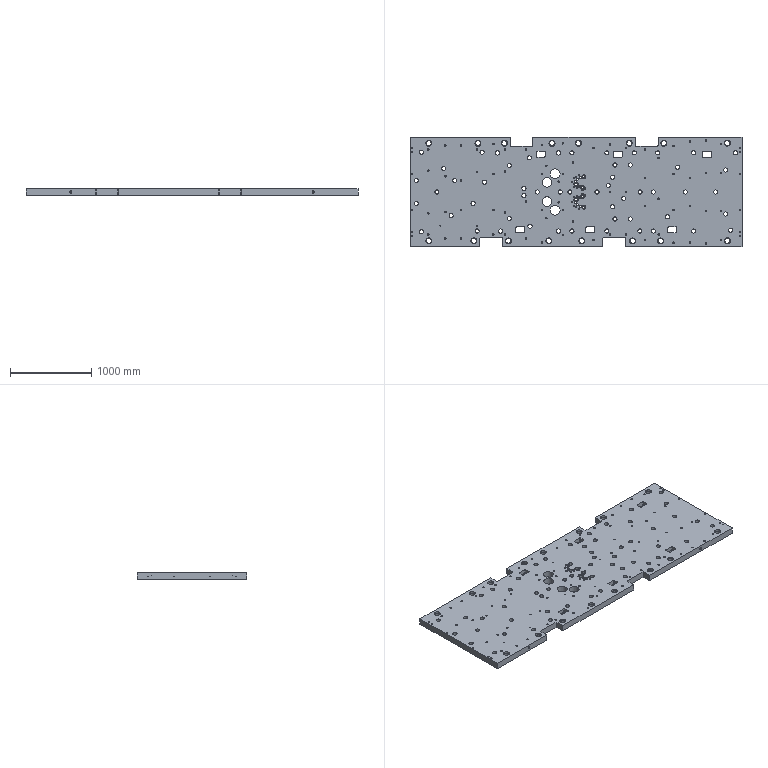Part | NX | features solid 2 | 1 solid | 1761 faces | box 4080 x 1345 x 80 mm | volume 396602174 mm3 | cylinder 932 | plane 418 | cone 411 | commonest cylinder face diameters 10.3 x169 8.5 x162 20 x84 18 x79 27 x79 10 x58